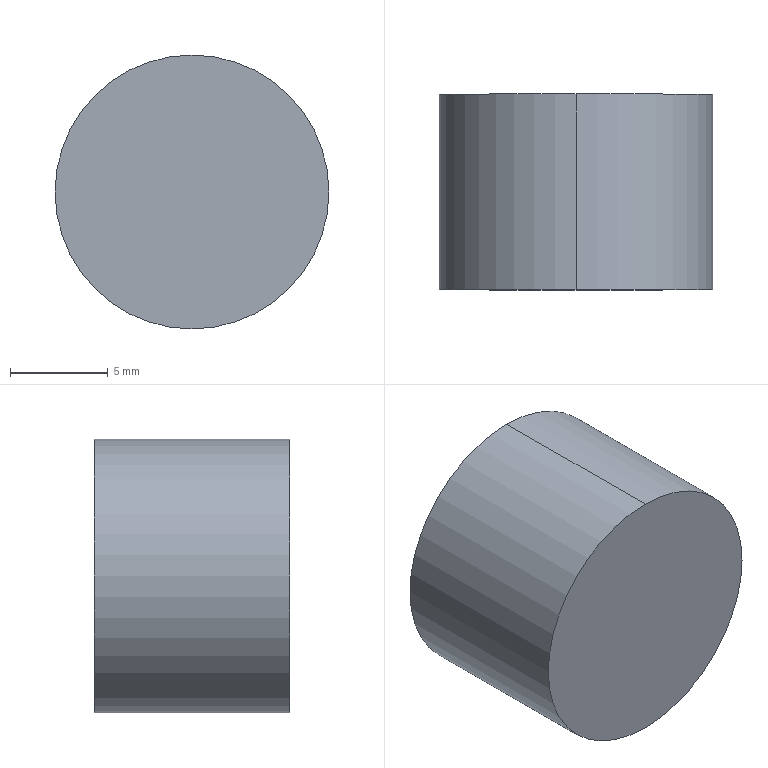Part | STEP file | OP10-126_seal pad dia7 | 1 solid | 4 faces | box 14 x 10 x 14 mm | volume 1539 mm3 | cylinder 2 | plane 2 | commonest cylinder face diameters 14 x2
STEP:
#1=CARTESIAN_POINT('',(0.,0.,0.));
#2=DIRECTION('',(0.,0.,1.));
#3=DIRECTION('',(1.,0.,0.));
#4=AXIS2_PLACEMENT_3D('',#1,#2,#3);
#5=CARTESIAN_POINT('',(0.,10.,7.));
#6=VERTEX_POINT('',#5);
#7=CARTESIAN_POINT('',(0.,10.,-7.));
#8=VERTEX_POINT('',#7);
#9=CARTESIAN_POINT('',(0.,10.,0.));
#10=DIRECTION('',(0.,1.,0.));
#11=DIRECTION('',(0.,0.,1.));
#12=AXIS2_PLACEMENT_3D('',#9,#10,#11);
#13=CIRCLE('',#12,7.);
#14=CARTESIAN_POINT('',(0.,10.,0.));
#15=DIRECTION('',(0.,-1.,0.));
#16=DIRECTION('',(0.,0.,-1.));
#17=AXIS2_PLACEMENT_3D('',#14,#15,#16);
#18=CYLINDRICAL_SURFACE('',#17,7.);
#19=CARTESIAN_POINT('',(3.142,0.));
#20=DIRECTION('',(-1.,0.));
#21=VECTOR('',#20,1.);
#22=LINE('',#19,#21);
#23=(GEOMETRIC_REPRESENTATION_CONTEXT(2)PARAMETRIC_REPRESENTATION_CONTEXT()REPRESENTATION_CONTEXT('',''));
#24=DEFINITIONAL_REPRESENTATION('',(#22),#23);
#25=PCURVE('',#18,#24);
#26=CARTESIAN_POINT('',(0.,10.,0.));
#27=DIRECTION('',(0.,1.,0.));
#28=DIRECTION('',(0.,0.,1.));
#29=AXIS2_PLACEMENT_3D('',#26,#27,#28);
#30=PLANE('',#29);
#31=CARTESIAN_POINT('',(0.,0.));
#32=DIRECTION('',(1.,0.));
#33=AXIS2_PLACEMENT_2D('',#31,#32);
#34=CIRCLE('',#33,7.);
#35=(GEOMETRIC_REPRESENTATION_CONTEXT(2)PARAMETRIC_REPRESENTATION_CONTEXT()REPRESENTATION_CONTEXT('',''));
#36=DEFINITIONAL_REPRESENTATION('',(#34),#35);
#37=PCURVE('',#30,#36);
#38=SURFACE_CURVE('',#13,(#25,#37),.PCURVE_S1.);
#39=EDGE_CURVE('',#6,#8,#38,.T.);
#40=ORIENTED_EDGE('',*,*,#39,.F.);
#41=CARTESIAN_POINT('',(0.,0.,7.));
#42=VERTEX_POINT('',#41);
#43=CARTESIAN_POINT('',(0.,10.,7.));
#44=DIRECTION('',(0.,-1.,0.));
#45=VECTOR('',#44,1.);
#46=LINE('',#43,#45);
#47=CARTESIAN_POINT('',(3.142,0.));
#48=DIRECTION('',(0.,1.));
#49=VECTOR('',#48,1.);
#50=LINE('',#47,#49);
#51=(GEOMETRIC_REPRESENTATION_CONTEXT(2)PARAMETRIC_REPRESENTATION_CONTEXT()REPRESENTATION_CONTEXT('',''));
#52=DEFINITIONAL_REPRESENTATION('',(#50),#51);
#53=PCURVE('',#18,#52);
#54=CARTESIAN_POINT('',(0.,10.,0.));
#55=DIRECTION('',(0.,-1.,0.));
#56=DIRECTION('',(0.,0.,-1.));
#57=AXIS2_PLACEMENT_3D('',#54,#55,#56);
#58=CYLINDRICAL_SURFACE('',#57,7.);
#59=CARTESIAN_POINT('',(3.142,0.));
#60=DIRECTION('',(0.,1.));
#61=VECTOR('',#60,1.);
#62=LINE('',#59,#61);
#63=(GEOMETRIC_REPRESENTATION_CONTEXT(2)PARAMETRIC_REPRESENTATION_CONTEXT()REPRESENTATION_CONTEXT('',''));
#64=DEFINITIONAL_REPRESENTATION('',(#62),#63);
#65=PCURVE('',#58,#64);
#66=SURFACE_CURVE('',#46,(#53,#65),.PCURVE_S1.);
#67=EDGE_CURVE('',#6,#42,#66,.T.);
#68=ORIENTED_EDGE('',*,*,#67,.T.);
#69=CARTESIAN_POINT('',(0.,0.,-7.));
#70=VERTEX_POINT('',#69);
#71=CARTESIAN_POINT('',(0.,0.,0.));
#72=DIRECTION('',(0.,1.,0.));
#73=DIRECTION('',(0.,0.,1.));
#74=AXIS2_PLACEMENT_3D('',#71,#72,#73);
#75=CIRCLE('',#74,7.);
#76=CARTESIAN_POINT('',(3.142,10.));
#77=DIRECTION('',(-1.,0.));
#78=VECTOR('',#77,1.);
#79=LINE('',#76,#78);
#80=(GEOMETRIC_REPRESENTATION_CONTEXT(2)PARAMETRIC_REPRESENTATION_CONTEXT()REPRESENTATION_CONTEXT('',''));
#81=DEFINITIONAL_REPRESENTATION('',(#79),#80);
#82=PCURVE('',#18,#81);
#83=CARTESIAN_POINT('',(0.,0.,0.));
#84=DIRECTION('',(0.,1.,0.));
#85=DIRECTION('',(0.,0.,1.));
#86=AXIS2_PLACEMENT_3D('',#83,#84,#85);
#87=PLANE('',#86);
#88=CARTESIAN_POINT('',(0.,0.));
#89=DIRECTION('',(1.,0.));
#90=AXIS2_PLACEMENT_2D('',#88,#89);
#91=CIRCLE('',#90,7.);
#92=(GEOMETRIC_REPRESENTATION_CONTEXT(2)PARAMETRIC_REPRESENTATION_CONTEXT()REPRESENTATION_CONTEXT('',''));
#93=DEFINITIONAL_REPRESENTATION('',(#91),#92);
#94=PCURVE('',#87,#93);
#95=SURFACE_CURVE('',#75,(#82,#94),.PCURVE_S1.);
#96=EDGE_CURVE('',#42,#70,#95,.T.);
#97=ORIENTED_EDGE('',*,*,#96,.T.);
#98=CARTESIAN_POINT('',(0.,10.,-7.));
#99=DIRECTION('',(0.,-1.,0.));
#100=VECTOR('',#99,1.);
#101=LINE('',#98,#100);
#102=CARTESIAN_POINT('',(0.,0.));
#103=DIRECTION('',(0.,1.));
#104=VECTOR('',#103,1.);
#105=LINE('',#102,#104);
#106=(GEOMETRIC_REPRESENTATION_CONTEXT(2)PARAMETRIC_REPRESENTATION_CONTEXT()REPRESENTATION_CONTEXT('',''));
#107=DEFINITIONAL_REPRESENTATION('',(#105),#106);
#108=PCURVE('',#18,#107);
#109=CARTESIAN_POINT('',(6.283,0.));
#110=DIRECTION('',(0.,1.));
#111=VECTOR('',#110,1.);
#112=LINE('',#109,#111);
#113=(GEOMETRIC_REPRESENTATION_CONTEXT(2)PARAMETRIC_REPRESENTATION_CONTEXT()REPRESENTATION_CONTEXT('',''));
#114=DEFINITIONAL_REPRESENTATION('',(#112),#113);
#115=PCURVE('',#58,#114);
#116=SURFACE_CURVE('',#101,(#108,#115),.PCURVE_S1.);
#117=EDGE_CURVE('',#8,#70,#116,.T.);
#118=ORIENTED_EDGE('',*,*,#117,.F.);
#119=EDGE_LOOP('',(#40,#68,#97,#118));
#120=FACE_BOUND('',#119,.T.);
#121=ADVANCED_FACE('',(#120),#18,.T.);
#122=ORIENTED_EDGE('',*,*,#67,.F.);
#123=CARTESIAN_POINT('',(0.,10.,0.));
#124=DIRECTION('',(0.,1.,0.));
#125=DIRECTION('',(0.,0.,1.));
#126=AXIS2_PLACEMENT_3D('',#123,#124,#125);
#127=CIRCLE('',#126,7.);
#128=CARTESIAN_POINT('',(9.425,0.));
#129=DIRECTION('',(-1.,0.));
#130=VECTOR('',#129,1.);
#131=LINE('',#128,#130);
#132=(GEOMETRIC_REPRESENTATION_CONTEXT(2)PARAMETRIC_REPRESENTATION_CONTEXT()REPRESENTATION_CONTEXT('',''));
#133=DEFINITIONAL_REPRESENTATION('',(#131),#132);
#134=PCURVE('',#58,#133);
#135=CARTESIAN_POINT('',(0.,0.));
#136=DIRECTION('',(1.,0.));
#137=AXIS2_PLACEMENT_2D('',#135,#136);
#138=CIRCLE('',#137,7.);
#139=(GEOMETRIC_REPRESENTATION_CONTEXT(2)PARAMETRIC_REPRESENTATION_CONTEXT()REPRESENTATION_CONTEXT('',''));
#140=DEFINITIONAL_REPRESENTATION('',(#138),#139);
#141=PCURVE('',#30,#140);
#142=SURFACE_CURVE('',#127,(#134,#141),.PCURVE_S1.);
#143=EDGE_CURVE('',#8,#6,#142,.T.);
#144=ORIENTED_EDGE('',*,*,#143,.F.);
#145=ORIENTED_EDGE('',*,*,#117,.T.);
#146=CARTESIAN_POINT('',(0.,0.,0.));
#147=DIRECTION('',(0.,1.,0.));
#148=DIRECTION('',(0.,0.,1.));
#149=AXIS2_PLACEMENT_3D('',#146,#147,#148);
#150=CIRCLE('',#149,7.);
#151=CARTESIAN_POINT('',(9.425,10.));
#152=DIRECTION('',(-1.,0.));
#153=VECTOR('',#152,1.);
#154=LINE('',#151,#153);
#155=(GEOMETRIC_REPRESENTATION_CONTEXT(2)PARAMETRIC_REPRESENTATION_CONTEXT()REPRESENTATION_CONTEXT('',''));
#156=DEFINITIONAL_REPRESENTATION('',(#154),#155);
#157=PCURVE('',#58,#156);
#158=CARTESIAN_POINT('',(0.,0.));
#159=DIRECTION('',(1.,0.));
#160=AXIS2_PLACEMENT_2D('',#158,#159);
#161=CIRCLE('',#160,7.);
#162=(GEOMETRIC_REPRESENTATION_CONTEXT(2)PARAMETRIC_REPRESENTATION_CONTEXT()REPRESENTATION_CONTEXT('',''));
#163=DEFINITIONAL_REPRESENTATION('',(#161),#162);
#164=PCURVE('',#87,#163);
#165=SURFACE_CURVE('',#150,(#157,#164),.PCURVE_S1.);
#166=EDGE_CURVE('',#70,#42,#165,.T.);
#167=ORIENTED_EDGE('',*,*,#166,.T.);
#168=EDGE_LOOP('',(#122,#144,#145,#167));
#169=FACE_BOUND('',#168,.T.);
#170=ADVANCED_FACE('',(#169),#58,.T.);
#171=ORIENTED_EDGE('',*,*,#143,.T.);
#172=ORIENTED_EDGE('',*,*,#39,.T.);
#173=EDGE_LOOP('',(#171,#172));
#174=FACE_BOUND('',#173,.T.);
#175=ADVANCED_FACE('',(#174),#30,.T.);
#176=ORIENTED_EDGE('',*,*,#166,.F.);
#177=ORIENTED_EDGE('',*,*,#96,.F.);
#178=EDGE_LOOP('',(#176,#177));
#179=FACE_BOUND('',#178,.T.);
#180=ADVANCED_FACE('',(#179),#87,.F.);
#181=CLOSED_SHELL('',(#121,#170,#175,#180));
#182=MANIFOLD_SOLID_BREP('',#181);
#183=(LENGTH_UNIT()NAMED_UNIT(*)SI_UNIT(.MILLI.,.METRE.));
#184=UNCERTAINTY_MEASURE_WITH_UNIT(LENGTH_MEASURE(0.0000001),#183,'','');
#185=(NAMED_UNIT(*)PLANE_ANGLE_UNIT()SI_UNIT($,.RADIAN.));
#186=(NAMED_UNIT(*)SI_UNIT($,.STERADIAN.)SOLID_ANGLE_UNIT());
#187=(GEOMETRIC_REPRESENTATION_CONTEXT(3)GLOBAL_UNCERTAINTY_ASSIGNED_CONTEXT((#184))GLOBAL_UNIT_ASSIGNED_CONTEXT((#183,#185,#186))REPRESENTATION_CONTEXT('',''));
#188=ADVANCED_BREP_SHAPE_REPRESENTATION('',(#4,#182),#187);